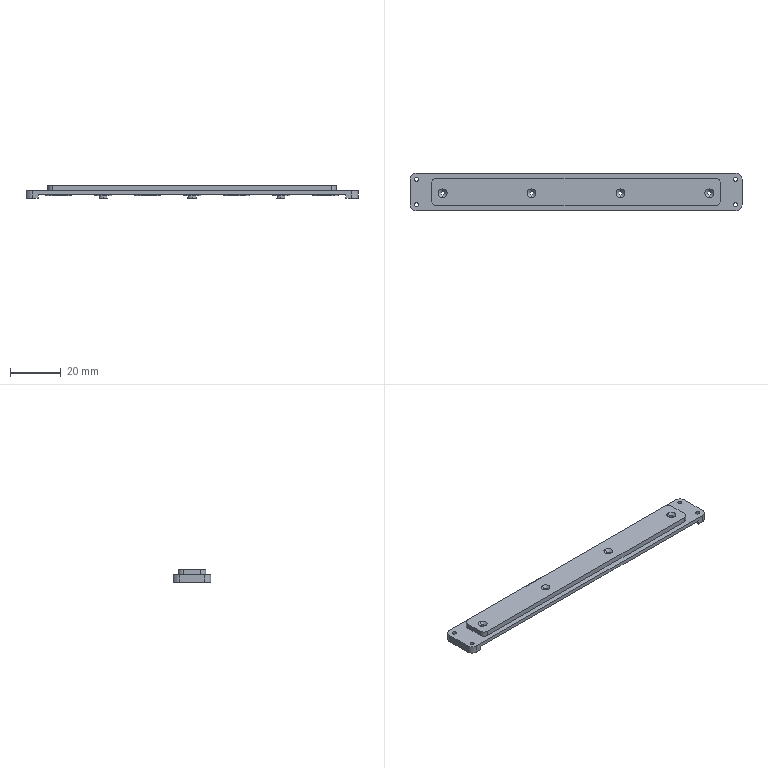NC program | NX | posted with a generic post | part box 130.666 x 14.95 x 5 mm
Whole program:
N10 G17 G21 G94 G90
(FLOOR_WALL_COPY , TOOL : D80)
N12 T19 M6
N14 G54
N16 G17 G0 G90 X-115.339 Y0. S6500 M3
N18 G43 Z30. H19
N20 Z3.
N22 G94 G1 Z0. F1500.
N24 X-110.339
N26 X110.327
N28 X115.327
N30 Z3.
N32 G0 Z30.
N34 M5
(DRILLING_COPY_1 , TOOL : D6A45)
N36 T01 M6
N38 G54
N40 G17 G0 G90 X62.827 Y4.975 S5000 M3
N42 G43 Z30. H1
N44 G94 G81 G98 Z-1.75 F350. R3.
N46 Y-4.975
N48 X52.5 Y-0.525
N50 X17.5
N52 X-17.5
N54 X-52.5
N56 X-62.839 Y-4.975
N58 Y4.975
N60 G80
N62 G0 X-62.839 Y4.975 Z30.
N64 M5
(DRILLING_COPY_1_COPY , TOOL : 1.5ZT)
N66 T16 M6
N68 G54
N70 G17 G0 G90 X-52.5 Y-0.525 S2000 M3
N72 G43 Z30. H16
N74 G94 G83 G98 Z-4.251 F100. Q2. R3.
N76 X-17.5
N78 X17.5
N80 X52.5
N82 G80
N84 G0 X52.5 Y-0.525 Z30.
N86 M5
(DRILLING_COPY_1_COPY_COPY , TOOL : 1.6ZT)
N88 T17 M6
N90 G54
N92 G17 G0 G90 X62.827 Y4.975 S2000 M3
N94 G43 Z30. H17
N96 G94 G83 G98 Z-6.981 F100. Q2. R3.
N98 Y-4.975
N100 X-62.839 Y4.975
N102 Y-4.975
N104 G80
N106 G0 X-62.839 Y-4.975 Z30.
N108 M5
(ADAPTIVE_MILLING , TOOL : D10)
N110 T15 M6
N112 G54
N114 G17 G0 G90 X-82.11 Y-0.024 S9500 M3
N116 G43 Z30. H15
N118 Z-2.
N120 G94 G1 Z-5. F1000.
N122 X-79.658 Y-1.424 F3000.
N124 G3 X-75.388 Y-0.024 R3.035
N126 X-74.737 Y3.235 R9.612
N128 X-74.527 Y10.23 R178.372
N130 G2 X-71.649 Y14.482 R6.101
N132 X-66.089 Y16.296 R13.045
N134 X-58.001 Y16.647 R72.901
N136 G1 X-56.601 Y16.655
N138 X-54.701 Y16.66
N140 X-51.601 Y16.664
N142 X-43.901 Y16.665
N144 X67.699
N146 X67.799 Y16.663
N148 G2 X72.245 Y13.949 R5.843
N150 X74.115 Y8.515 R12.405
N152 X74.502 Y-0.17 R71.821
N154 X74.488 Y-10.269 R480.831
N156 X71.513 Y-14.563 R6.095
N158 X65.83 Y-16.325 R13.532
N160 X56.84 Y-16.656 R85.511
N162 G1 X54.84 Y-16.661
N164 X51.44 Y-16.664
N166 X41.74 Y-16.665
N168 X-67.66
N170 X-67.76 Y-16.664
N172 X-67.86 Y-16.66
N174 G2 X-72.276 Y-13.889 R5.908
N176 X-74.129 Y-8.448 R12.646
N178 X-74.166 Y0.826 R34.955
N180 G3 X-73.763 Y7.812 R172.113
N182 G2 X-69.669 Y13.647 R7.849
N184 X-63.378 Y15.484 R16.244
N186 X-53.789 Y15.842 R94.409
N188 G1 X-52.089 Y15.848
N190 X-49.689 Y15.853
N192 X-45.489 Y15.856
N194 X-25.789 Y15.857
N196 X64.911
N198 X65.011 Y15.856
N200 G2 X71.329 Y12.063 R7.559
N202 X73.298 Y5.817 R15.364
N204 X73.691 Y-3.469 R83.486
N206 X73.657 Y-7.867 R68.82
N208 X69.632 Y-13.633 R7.757
N210 X63.245 Y-15.494 R16.332
N212 X53.657 Y-15.853 R95.773
N214 G1 X51.757 Y-15.861
N216 X48.457 Y-15.867
N218 X45.457
N220 X42.757 Y-15.869
N222 X39.757 Y-15.866
N224 X36.757 Y-15.868
N226 X35.257 Y-15.869
N228 X32.257 Y-15.866
N230 X29.257 Y-15.867
N232 X27.657 Y-15.869
N234 X24.657 Y-15.866
N236 X21.657 Y-15.867
N238 X20.057 Y-15.869
N240 X17.057 Y-15.866
N242 X14.057 Y-15.867
N244 X12.457 Y-15.869
N246 X9.457 Y-15.866
N248 X6.457 Y-15.867
N250 X4.857 Y-15.869
N252 X1.857 Y-15.866
N254 X-1.143 Y-15.867
N256 X-2.743 Y-15.869
N258 X-5.743 Y-15.866
N260 X-8.743 Y-15.867
N262 X-10.343 Y-15.869
N264 X-13.343 Y-15.866
N266 X-16.343 Y-15.868
N268 X-17.843 Y-15.869
N270 X-20.843 Y-15.866
N272 X-23.843 Y-15.867
N274 X-25.543 Y-15.869
N276 X-28.543 Y-15.866
N278 X-31.543 Y-15.867
N280 X-33.143 Y-15.869
N282 X-36.143 Y-15.866
N284 X-39.143 Y-15.868
N286 X-40.643 Y-15.869
N288 X-43.643 Y-15.866
N290 X-46.643 Y-15.867
N292 X-48.243 Y-15.869
N294 X-51.243 Y-15.866
N296 X-54.243 Y-15.867
N298 X-55.843 Y-15.869
N300 X-58.843 Y-15.866
N302 G2 X-65.742 Y-15.818 R126.962
N304 X-71.45 Y-11.868 R7.738
N306 X-73.359 Y-5.294 R15.946
N308 X-73.289 Y1.099 R43.284
N310 X-72.978 Y6.188 R89.038
N312 X-67.955 Y12.88 R9.064
N314 X-61.331 Y14.665 R18.69
N316 X-51.642 Y15.029 R102.154
N318 G1 X-50.042 Y15.037
N320 X-47.942 Y15.042
N322 X-44.742 Y15.046
N324 X-37.642 Y15.048
N326 X62.558
N328 X62.858 Y15.044
N330 G2 X70.616 Y10.235 R8.787
N332 X72.506 Y3.541 R18.063
N334 X72.822 Y-5.846 R70.946
N336 X68.025 Y-12.783 R8.784
N338 X61.228 Y-14.673 R18.294
N340 X51.139 Y-15.043 R105.617
N342 G1 X49.639 Y-15.05
N344 X47.339 Y-15.054
N346 X46.039 Y-15.057
N348 X43.539 Y-15.067
N350 X40.539 Y-15.068
N352 X37.939 Y-15.072
N354 X34.739 Y-15.07
N356 X31.639 Y-15.072
N358 X30.339 Y-15.073
N360 X27.139 Y-15.07
N362 X24.039
N364 X21.839 Y-15.072
N366 X18.639 Y-15.068
N368 X15.539 Y-15.069
N370 X13.039 Y-15.071
N372 X10.039 Y-15.068
N374 X7.039 Y-15.069
N376 X5.339 Y-15.071
N378 X2.339 Y-15.068
N380 X-0.661 Y-15.069
N382 X-2.261 Y-15.071
N384 X-5.261 Y-15.068
N386 X-8.261 Y-15.069
N388 X-9.861 Y-15.071
N390 X-12.861 Y-15.068
N392 X-15.861 Y-15.069
N394 X-17.461 Y-15.071
N396 X-20.461 Y-15.068
N398 X-23.461 Y-15.069
N400 X-25.061 Y-15.071
N402 X-28.061 Y-15.068
N404 X-31.061 Y-15.069
N406 X-32.661 Y-15.071
N408 X-35.661 Y-15.068
N410 X-38.661 Y-15.069
N412 X-40.161 Y-15.071
N414 X-43.161 Y-15.068
N416 X-46.161 Y-15.069
N418 X-47.861 Y-15.071
N420 X-50.861 Y-15.068
N422 X-53.861 Y-15.069
N424 X-55.361 Y-15.071
N426 X-58.361 Y-15.068
N428 G2 X-63.759 Y-15.008 R83.437
N430 X-70.569 Y-10.332 R8.808
N432 X-72.416 Y-3.032 R16.267
N434 X-72.207 Y4.558 R54.045
N436 X-66.798 Y11.918 R9.847
N438 X-59.596 Y13.847 R20.024
N440 X-48.007 Y14.226 R125.517
N442 G1 X-45.907 Y14.233
N444 X-42.807 Y14.237
N446 X-37.007 Y14.239
N448 X60.493
N450 X60.793 Y14.236
N452 X61.093 Y14.23
N454 G2 X69.781 Y8.8 R9.65
N456 X71.675 Y1.897 R19.464
N458 X71.924 Y-4.39 R35.825
N460 X66.73 Y-11.869 R9.489
N462 X59.743 Y-13.823 R19.22
N464 X49.855 Y-14.227 R99.699
N466 G1 X47.955 Y-14.238
N468 X44.655 Y-14.253
N470 X41.355 Y-14.264
N472 X38.055 Y-14.271
N474 X34.755 Y-14.275
N476 X31.455
N478 X28.155 Y-14.271
N480 X26.555 Y-14.268
N482 X23.355 Y-14.27
N484 X20.255 Y-14.267
N486 X18.755 Y-14.265
N488 X15.555 Y-14.268
N490 X12.455 Y-14.266
N492 X10.655 Y-14.264
N494 X7.455 Y-14.268
N496 X4.355 Y-14.267
N498 X2.155 Y-14.265
N500 X-1.045 Y-14.268
N502 X-4.145
N504 X-6.345 Y-14.266
N506 X-9.545 Y-14.269
N508 X-12.645
N510 X-15.445 Y-14.266
N512 X-18.445 Y-14.269
N514 X-21.445 Y-14.268
N516 X-23.445 Y-14.266
N518 X-26.445 Y-14.268
N520 X-29.445 Y-14.267
N522 X-30.945 Y-14.265
N524 X-33.945 Y-14.269
N526 X-36.945 Y-14.268
N528 X-39.345 Y-14.265
N530 X-42.345 Y-14.267
N532 X-45.345 Y-14.266
N534 X-46.445 Y-14.265
N536 X-49.445 Y-14.268
N538 G2 X-61.544 Y-14.233 R740.642
N540 X-69.927 Y-8.496 R9.64
N542 X-71.453 Y-1.609 R18.215
N544 X-71.223 Y3.971 R21.952
N546 X-70.303 Y6.613 R15.353
N548 G1 X-70.292 Y6.676
N550 X-70.269 Y6.758
N552 X-69.76 Y8.213
N554 X-69.727 Y8.292
N556 X-69.686 Y8.367
N558 G2 X-67.669 Y10.895 R8.648
N560 G1 X-67.606 Y10.952
N562 X-67.536 Y11.002
N564 X-66.231 Y11.822
N566 X-66.156 Y11.863
N568 X-66.077 Y11.896
N570 G2 X-62.924 Y12.615 R8.648
N572 X-49.257 Y13.401 R101.16
N574 G1 X-48.057 Y13.41
N576 X-46.257 Y13.418
N578 X-43.957 Y13.424
N580 X-40.557 Y13.428
N582 X-33.957 Y13.43
N584 X58.543
N586 X58.943 Y13.427
N588 X59.143 Y13.424
N590 X59.442 Y13.416
N592 X59.642 Y13.409
N594 G2 X63.929 Y12.524 R13.015
N596 X66.219 Y11.822 R8.86
N598 X68.748 Y9.805 R8.648
N600 G1 X68.805 Y9.742
N602 X68.854 Y9.672
N604 X69.674 Y8.367
N606 X69.715 Y8.292
N608 X69.748 Y8.213
N610 G2 X70.468 Y5.06 R8.648
N612 X71.044 Y-2.51 R47.845
N614 X70.379 Y-5.845 R14.708
N616 G1 X70.295 Y-6.592
N618 X70.281 Y-6.676
N620 X70.257 Y-6.758
N622 G2 X68.854 Y-9.672 R8.648
N624 G1 X68.805 Y-9.742
N626 X68.748 Y-9.805
N628 X67.658 Y-10.896
N630 X67.594 Y-10.952
N632 X67.525 Y-11.002
N634 G2 X64.61 Y-12.405 R8.648
N636 X48.346 Y-13.42 R110.576
N638 G1 X46.346 Y-13.433
N640 X43.946 Y-13.444
N642 X40.946 Y-13.455
N644 X37.746 Y-13.462
N646 X34.546 Y-13.465
N648 X31.346
N650 X29.146 Y-13.463
N652 X25.946 Y-13.468
N654 X22.846
N656 X19.746 Y-13.465
N658 X19.146 Y-13.464
N660 X15.946 Y-13.467
N662 X12.846 Y-13.465
N664 X11.046 Y-13.463
N666 X7.846 Y-13.467
N668 X4.746 Y-13.466
N670 X2.546 Y-13.464
N672 X-0.654 Y-13.467
N674 X-3.754
N676 X-5.954 Y-13.464
N678 X-9.154 Y-13.468
N680 X-12.254
N682 X-15.054 Y-13.465
N684 X-18.254 Y-13.468
N686 X-21.354 Y-13.467
N688 X-23.654 Y-13.464
N690 X-26.854 Y-13.468
N692 X-29.954 Y-13.467
N694 X-32.054 Y-13.465
N696 X-35.254 Y-13.468
N698 X-38.354
N700 X-41.554 Y-13.464
N702 X-44.554 Y-13.466
N704 X-47.454 Y-13.464
N706 X-47.754
N708 X-50.754 Y-13.468
N710 X-53.754 Y-13.467
N712 X-56.854 Y-13.464
N714 X-58.254 Y-13.465
N716 X-58.554 Y-13.464
N718 X-58.854 Y-13.46
N720 X-59.254 Y-13.452
N722 X-59.553 Y-13.442
N724 G2 X-64.032 Y-12.51 R13.921
N726 X-66.231 Y-11.822 R8.956
N728 X-68.759 Y-9.805 R8.648
N730 G1 X-68.816 Y-9.742
N732 X-68.865 Y-9.672
N734 X-69.686 Y-8.367
N736 X-69.727 Y-8.292
N738 X-69.76 Y-8.213
N740 G2 X-70.479 Y-5.06 R8.648
N742 X-70.576 Y1.305 R48.451
N744 G1 X-70.555 Y1.504
N746 X-70.544 Y1.603
N748 X-70.52 Y1.802
N750 X-70.506 Y1.901
N752 X-70.496 Y2.
N754 X-70.489 Y2.1
N756 Y4.889
N758 X-70.479 Y5.06
N760 X-70.307 Y6.592
N762 X-70.292 Y6.676
N764 X-69.727 Y8.292
N766 X-68.816 Y9.742
N768 X-67.606 Y10.952
N770 X-66.156 Y11.863
N772 X-64.54 Y12.429
N774 X-62.924 Y12.615
N776 X-62.753 Y12.625
N778 X62.742
N780 X62.912 Y12.615
N782 X64.204 Y12.47
N784 X64.61 Y12.405
N786 X66.144 Y11.863
N788 X67.594 Y10.952
N790 X68.805 Y9.742
N792 X69.715 Y8.292
N794 X70.281 Y6.676
N796 X70.468 Y5.06
N798 X70.477 Y4.889
N800 Y-4.889
N802 X70.468 Y-5.06
N804 X70.378 Y-5.855
N806 X70.333 Y-6.309
N808 X70.257 Y-6.758
N810 X69.715 Y-8.292
N812 X68.805 Y-9.742
N814 X67.594 Y-10.952
N816 X66.144 Y-11.863
N818 X64.529 Y-12.429
N820 X62.912 Y-12.615
N822 X62.742 Y-12.625
N824 X-62.753
N826 X-62.924 Y-12.615
N828 X-64.315 Y-12.459
N830 X-64.622 Y-12.405
N832 X-66.156 Y-11.863
N834 X-67.606 Y-10.952
N836 X-68.816 Y-9.742
N838 X-69.727 Y-8.292
N840 X-70.292 Y-6.676
N842 X-70.489 Y-4.889
N844 Y2.111
N846 G3 X-73.76 Y5.131 R3.035
N848 G1 X-76.789 Y4.889
N850 Z-2.
N852 G0 Z30.
N854 X-77.211 Y-0.025
N856 Z1.151
N858 G1 Z-1.849 F1000.
N860 X-74.759 Y-1.424 F3000.
N862 G3 X-70.489 Y-0.025 R3.035
N864 X-69.87 Y2.836 R8.796
N866 G2 X-68.369 Y7.646 R9.787
N868 X-63.549 Y10.844 R8.602
N870 X-56.918 Y11.678 R27.764
N872 X-37.619 Y11.766 R862.53
N874 G1 X60.281
N876 X60.381 Y11.765
N878 X60.581 Y11.762
N880 X60.881 Y11.752
N882 G2 X66.581 Y9.485 R7.949
N884 X68.997 Y4.407 R10.108
N886 X69.473 Y-4.257 R34.959
N888 X64.497 Y-10.477 R7.496
N890 X58.226 Y-11.612 R20.249
N892 X46.329 Y-11.764 R277.088
N894 G1 X39.429 Y-11.766
N896 X-60.271
N898 X-60.471 Y-11.764
N900 X-60.771 Y-11.756
N902 X-60.971 Y-11.748
N904 G2 X-66.644 Y-9.424 R7.855
N906 X-69.057 Y-4.126 R10.496
N908 X-69.091 Y1.658 R23.105
N910 X-63.866 Y9.133 R8.694
N912 X-57.083 Y10.702 R19.705
N914 X-45.989 Y10.952 R155.335
N916 G1 X-42.889 Y10.955
N918 X-35.689 Y10.957
N920 X58.311
N922 X58.611 Y10.955
N924 X58.811 Y10.951
N926 X59.111 Y10.943
N928 G2 X66.831 Y6.156 R8.359
N930 X68.485 Y-2.789 R17.968
N932 X64.19 Y-8.822 R8.018
N934 X57.779 Y-10.608 R16.868
N936 X48.389 Y-10.943 R98.447
N938 G1 X46.689 Y-10.949
N940 X44.289 Y-10.954
N942 X39.889 Y-10.957
N944 X13.089
N946 X-58.211
N948 X-58.611 Y-10.954
N950 G2 X-63.601 Y-9.761 R9.277
N952 X-67.723 Y-3.508 R9.506
N954 X-67.746 Y2.336 R12.462
N956 X-62.596 Y8.136 R9.335
N958 X-58.811 Y9.406 R21.047
N960 G3 X-57.796 Y9.945 R13.038
N962 G2 X-54.689 Y10.625 R8.25
N964 G1 X54.689
N966 X54.86 Y10.615
N968 G2 X59.551 Y10.026 R57.234
N970 X65.987 Y4.63 R9.526
N972 X67.284 Y-1.165 R12.054
N974 X63.18 Y-7.566 R8.297
N976 X59.03 Y-9.259 R15.444
N978 G3 X57.796 Y-9.945 R15.628
N980 G2 X54.689 Y-10.625 R8.25
N982 G1 X-54.689
N984 X-54.86 Y-10.615
N986 G2 X-59.551 Y-10.027 R56.99
N988 X-66.136 Y-3.907 R9.155
N990 X-62.799 Y6.292 R8.55
N992 G1 X-60.756 Y7.547
N994 X-60.679 Y7.61
N996 X-60.604 Y7.676
N998 X-60.531 Y7.744
N1000 X-60.459 Y7.815
N1002 X-60.412 Y7.858
N1004 X-60.361 Y7.93
N1006 X-60.305 Y7.993
N1008 X-59.293 Y9.005
N1010 X-59.23 Y9.061
N1012 X-59.16 Y9.111
N1014 X-58.398 Y9.589
N1016 G3 X-57.231 Y10.963 R3.044
N1018 X-57.232 Y13.3 Z-1.749 R3.031
N1020 X-61.87 Y14.471 R3.004
N1022 G1 X-69.157 Y8.635
N1024 G3 X-70.279 Y6.406 R3.023
N1026 G1 X-70.378 Y3.846
N1028 X-70.459 Y1.285
N1030 G3 X-70.264 Y-1.695 R22.722
N1032 G1 X-69.977 Y-3.545
N1034 X-69.633 Y-5.385
N1036 X-68.581 Y-10.455
N1038 G3 X-66.764 Y-12.629 R3.018
N1040 G1 X-57.904 Y-16.196
N1042 G3 X-53.795 Y-13.68 R3.003
N1044 X-54.51 Y-11.456 Z-1.849 R3.031
N1046 X-56.281 Y-10.455 R3.042
N1048 G2 X-61.267 Y-8.194 R17.096
N1050 X-65.036 Y-1.864 R8.819
N1052 X-62.872 Y4.08 R8.123
N1054 G3 X-61.55 Y5.703 R9.51
N1056 G2 X-60.411 Y7.86 R8.158
N1058 G3 X-59.951 Y9.412 R3.071
N1060 X-60.829 Y11.578 Z-1.749 R3.031
N1062 X-65.806 Y10.377 R3.003
N1064 G1 X-68.992 Y0.499
N1066 G3 X-69.108 Y-0.837 R3.106
N1068 G1 X-68.054 Y-8.385
N1070 G3 X-66.939 Y-10.327 R3.032
N1072 G1 X-60.741 Y-15.208
N1074 G3 X-56.369 Y-14.486 R3.005
N1076 X-55.96 Y-12.185 Z-1.849 R3.031
N1078 G1 X-56.05 Y-11.871
N1080 X-56.173 Y-11.569
N1082 G3 X-57.95 Y-9.871 R3.13
N1084 G2 X-60.813 Y-7.556 R10.961
N1086 X-63.323 Y-2.056 R8.058
N1088 X-62.136 Y2.551 R10.547
N1090 G3 X-61.915 Y3.56 R4.467
N1092 G1 X-61.755 Y4.981
N1094 X-61.741 Y5.065
N1096 X-61.717 Y5.147
N1098 X-61.42 Y5.996
N1100 G3 X-61.333 Y7.884 R3.349
N1102 X-62.674 Y9.811 Z-1.749 R3.335
N1104 X-67.795 Y6.572 R3.302
N1106 G1 X-64.887 Y-11.853
N1108 G3 X-58.699 Y-12.861 R3.301
N1110 X-58.428 Y-10.529 Z-1.849 R3.335
N1112 X-59.293 Y-9.005 R3.376
N1114 G2 X-61.717 Y-5.147 R7.584
N1116 X-61.925 Y-1.337 R10.363
N1118 G1 Y3.363
N1120 G3 X-62.474 Y5.186 R3.349
N1122 X-64.382 Y6.554 Z-1.749 R3.335
N1124 X-68.524 Y3.279 R3.304
N1126 G1 X-68.293 Y-5.702
N1128 G3 X-63.546 Y-8.583 R3.303
N1130 X-61.941 Y-6.87 Z-1.849 R3.335
N1132 X-61.741 Y-5.065 R3.35
N1134 G2 X-61.925 Y-1.289 R20.766
N1136 G3 X-62.413 Y0.351 R3.046
N1138 G1 X-63.552 Y2.094
N1140 X-64.864 Y4.103 Z-1.749
N1142 X-66.278 Y6.267
N1144 G2 X-65.108 Y10.591 R3.005
N1146 G1 X-63.293 Y11.5
N1148 X-61.469 Y12.394
N1150 G2 X-58.275 Y13.631 R26.965
N1152 X-55.22 Y14.105 R12.33
N1154 G1 X19. Y15.965
N1156 X45.629 Y16.605
N1158 G2 X47.367 Y16.1 R3.044
N1160 G1 X51.052 Y13.636
N1162 X53.047 Y12.302 Z-1.849
N1164 X55.116 Y10.919
N1166 G3 X56.281 Y10.455 R3.112
N1168 G2 X61.437 Y8.09 R17.397
N1170 X65.737 Y1.125 R10.625
N1172 X62.451 Y-6.086 R7.933
N1174 G3 X60.849 Y-7.278 R16.749
N1176 G2 X59.16 Y-9.111 R11.078
N1178 G1 X58.568 Y-9.483
N1180 G3 X57.38 Y-10.906 R3.044
N1182 X57.423 Y-13.242 Z-1.749 R3.031
N1184 X62.654 Y-13.697 R3.002
N1186 G1 X68.73 Y-4.658
N1188 G3 X69.22 Y-3.333 R3.081
N1190 X69.537 Y0.383 R36.911
N1192 G1 X69.677 Y6.762
N1194 G3 X68.496 Y9.215 R3.018
N1196 G1 X60.762 Y15.104
N1198 G3 X56.062 Y13.549 R3.003
N1200 X56.34 Y11.229 Z-1.849 R3.031
N1202 X57.796 Y9.945 R3.043
N1204 G2 X60.696 Y7.723 R11.341
N1206 X63.8 Y3.133 R11.221
N1208 X62.706 Y-3.348 R7.584
N1210 G3 X61.717 Y-5.147 R5.854
N1212 G2 X60.533 Y-7.666 R7.653
N1214 G3 X60.028 Y-9.37 R3.376
N1216 X60.828 Y-11.577 Z-1.749 R3.335
N1218 X66.616 Y-9.152 R3.301
N1220 G1 X64.916 Y11.607
N1222 G3 X58.7 Y12.861 R3.301
N1224 X58.427 Y10.53 Z-1.849 R3.335
N1226 X59.293 Y9.005 R3.376
N1228 G2 X61.213 Y6.575 R8.136
N1230 X62.116 Y-1.115 R9.076
N1232 G3 X61.925 Y-3.389 R6.779
N1234 G1 X61.915 Y-3.56
N1236 X61.755 Y-4.981
N1238 X61.741 Y-5.065
N1240 G3 X61.919 Y-6.814 R3.376
N1242 X63.493 Y-8.556 Z-1.749 R3.335
N1244 X68.29 Y-5.438 R3.302
N1246 G1 X67.557 Y8.018
N1248 G3 X62.191 Y10.408 R3.302
N1250 X61.006 Y8.381 Z-1.849 R3.335
N1252 X61.213 Y6.575 R3.35
N1254 G2 X61.925 Y3.389 R8.29
N1256 G1 Y-2.111
N1258 G3 X65.161 Y-5.134 R3.035
N1260 G1 X68.096 Y-4.934
N1262 Z1.151
N1264 G0 Z30.
N1266 M5
(ZLEVEL_PROFILE_COPY_1_COPY_COPY_1 , TOOL : D10JING)
N1268 T14 M6
N1270 G54
N1272 G17 G0 G90 X-64.488 Y14.331 S9500 M3
N1274 G43 Z30. H14
N1276 Z-4.
N1278 G94 G1 Z-5. F1000.
N1280 X-63.705 Y12.975
N1282 G3 X-62.839 Y12.475 R1.
N1284 G1 X62.827 F1200.
N1286 G2 X70.327 Y4.975 R7.5
N1288 G1 Y-4.975
N1290 G2 X62.827 Y-12.475 R7.5
N1292 G1 X-62.839
N1294 G2 X-70.339 Y-4.975 R7.5
N1296 G1 Y4.975
N1298 G2 X-62.839 Y12.475 R7.5
N1300 G3 X-61.973 Y12.975 R1.
N1302 G1 X-61.107 Y14.475
N1304 Z-4.
N1306 G0 Z30.
(ZLEVEL_PROFILE_COPY_1_COPY_COPY_1_COPY , TOOL : D10JING)
N1308 X56.42 Y-12.323
N1310 Z-1.
N1312 G1 Z-2. F1000.
N1314 X55.641 Y-10.975
N1316 G3 X54.775 Y-10.475 R1.
N1318 G1 X-54.775 F1200.
N1320 G2 X-61.775 Y-3.475 R7.
N1322 G1 Y3.475
N1324 G2 X-54.775 Y10.475 R7.
N1326 G1 X54.775
N1328 G2 X61.775 Y3.475 R7.
N1330 G1 Y-3.475
N1332 G2 X54.775 Y-10.475 R7.
N1334 G3 X53.909 Y-10.975 R1.
N1336 G1 X53.043 Y-12.475
N1338 Z-1.
N1340 G0 Z30.
N1342 M5
(PLANAR_MILL_COPY_COPY_COPY_COPY_COPY_COPY_1 , TOOL : D6A45)
N1344 T01 M6
N1346 G54
N1348 G17 G0 G90 X1.27 Y-7.575 S9500 M3
N1350 G43 Z30. H1
N1352 Z0.5
N1354 G94 G1 Z-1. F1250.
N1356 X0.866 Y-6.875
N1358 G3 X0. Y-6.375 R1.
N1360 G1 X-54.775
N1362 G2 X-57.675 Y-3.475 R2.9
N1364 G1 Y3.475
N1366 G2 X-54.775 Y6.375 R2.9
N1368 G1 X54.775
N1370 G2 X57.675 Y3.475 R2.9
N1372 G1 Y-3.475
N1374 G2 X54.775 Y-6.375 R2.9
N1376 G1 X0.
N1378 G3 X-0.866 Y-6.875 R1.
N1380 G1 X-1.27 Y-7.575
N1382 Z0.5
N1384 G0 Z30.
(PLANAR_MILL_COPY_COPY_COPY_COPY_COPY_COPY_1_COPY , TOOL : D6A45)
N1386 X-1.276 Y11.075
N1388 Z-3.
N1390 G1 Z-4.5
N1392 X-0.872 Y10.375
N1394 G3 X-0.006 Y9.875 R1.
N1396 G1 X62.827
N1398 G2 X67.727 Y4.975 R4.9
N1400 G1 Y-4.975
N1402 G2 X62.827 Y-9.875 R4.9
N1404 G1 X-62.839
N1406 G2 X-67.739 Y-4.975 R4.9
N1408 G1 Y4.975
N1410 G2 X-62.839 Y9.875 R4.9
N1412 G1 X-0.006
N1414 G3 X0.86 Y10.375 R1.
N1416 G1 X1.264 Y11.075
N1418 Z-3.
N1420 G0 Z30.
(DRILLING_COPY_1_COPY_1 , TOOL : D6A45)
N1422 X62.827 Y4.975 S5000
N1424 G81 G98 Z-3.1 F350. R1.
N1426 Y-4.975
N1428 X-62.839
N1430 Y4.975
N1432 G80
N1434 G0 X-62.839 Y4.975 Z30.
N1436 M5
N1438 M2